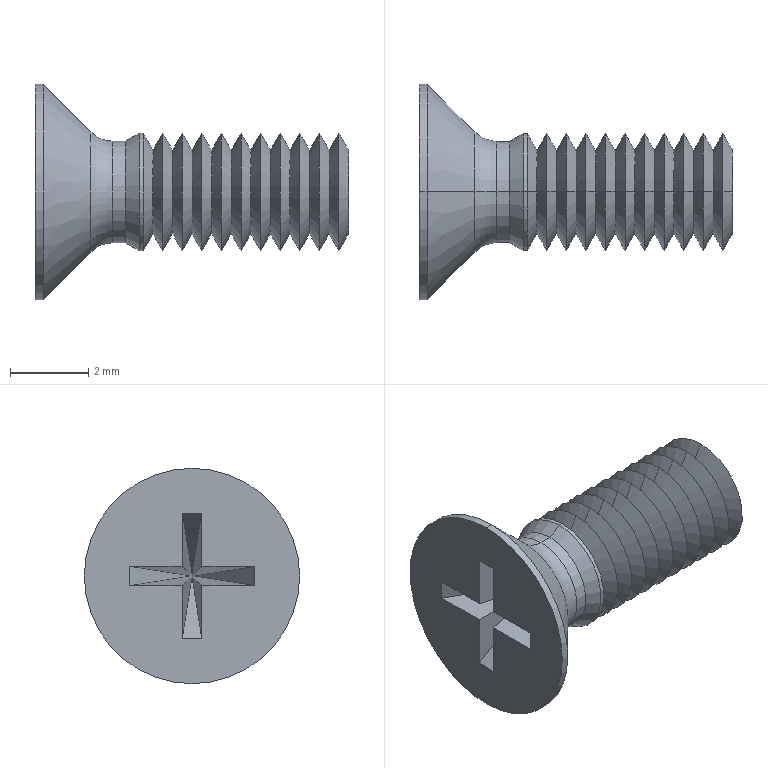Part | STEP file | 1 solid | 68 faces | box 8 x 5.5 x 5.5 mm | volume 56.004 mm3 | cone 46 | plane 14 | cylinder 6 | torus 2 | commonest cylinder face diameters 2.598 x2 3 x2 5.5 x2